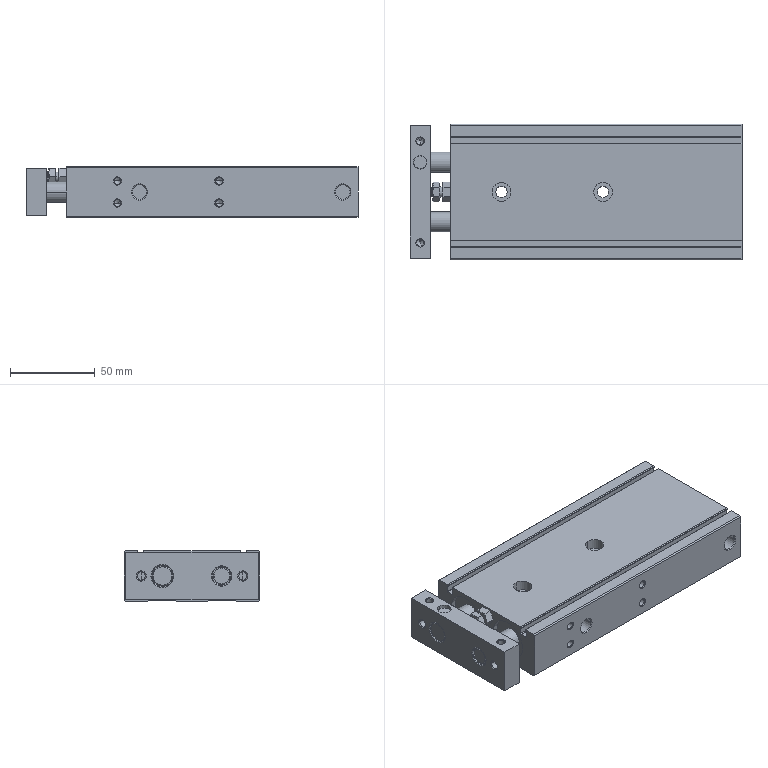Part | STEP file | 2 solids | 275 faces | box 196 x 80 x 30 mm | volume 343532 mm3 | cone 100 | cylinder 98 | plane 77 | commonest cylinder face diameters 4.134 x20 0.8 x12 25 x12 12 x10 8.566 x8 11 x6